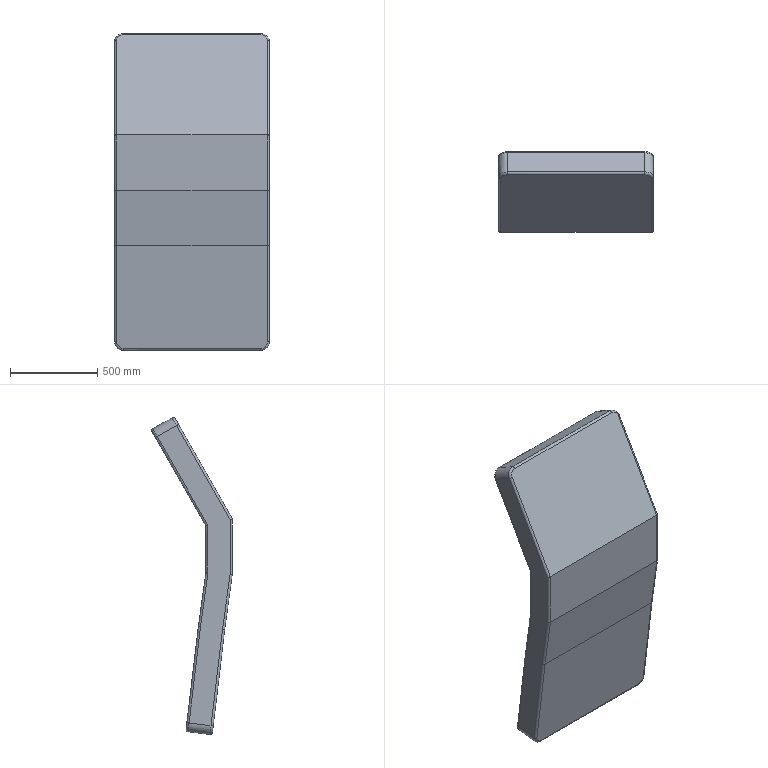Part | NX | features BREP 1 | 1 solid | 44 faces | box 889 x 462.14 x 1820 mm | volume 252935274 mm3 | cylinder 24 | plane 12 | torus 8 | commonest cylinder face diameters 25.4 x20 101.6 x4